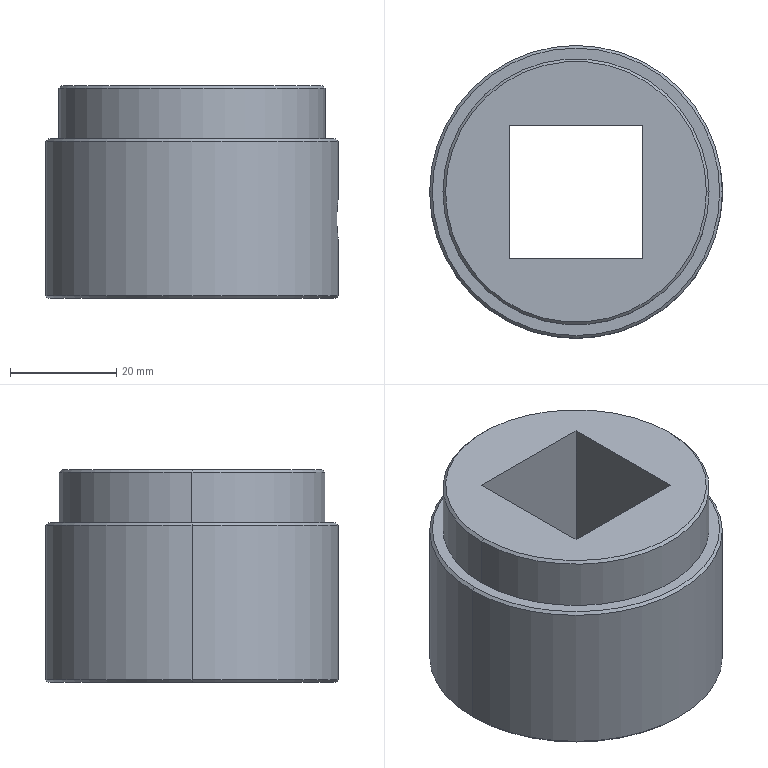Part | STEP file | BCC3 H16_7 | 1 solid | 21 faces | box 55 x 55 x 40 mm | volume 65270 mm3 | plane 7 | cone 6 | cylinder 6 | spline 2 | commonest cylinder face diameters 7 x2 50 x2 55 x2